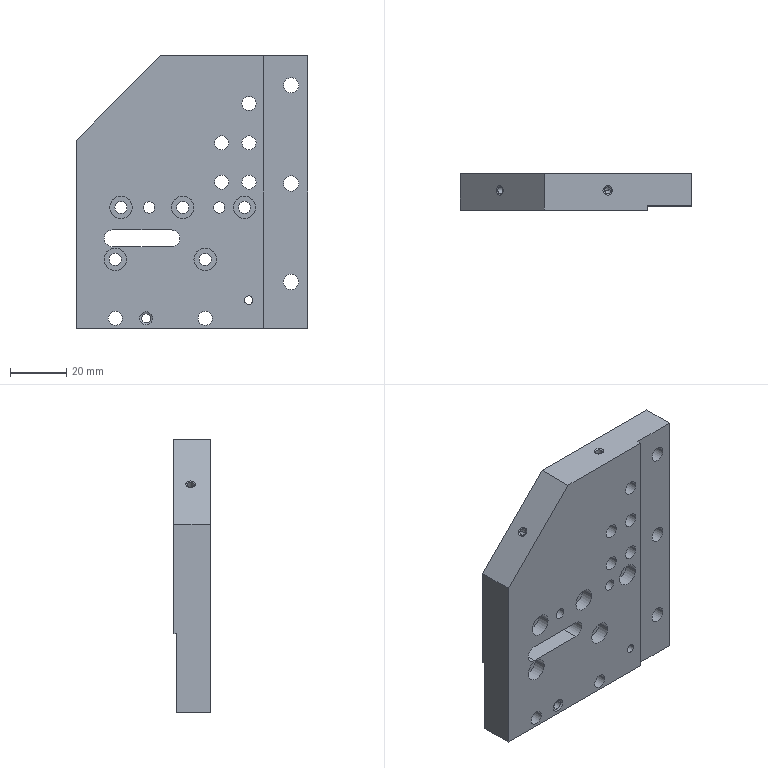Part | NX | 1 solid | 92 faces | box 82.6 x 13 x 97 mm | volume 85868 mm3 | cylinder 61 | plane 21 | cone 10 | commonest cylinder face diameters 5 x14 4.3 x10 8 x10 5.5 x6 10 x6 2.5 x4